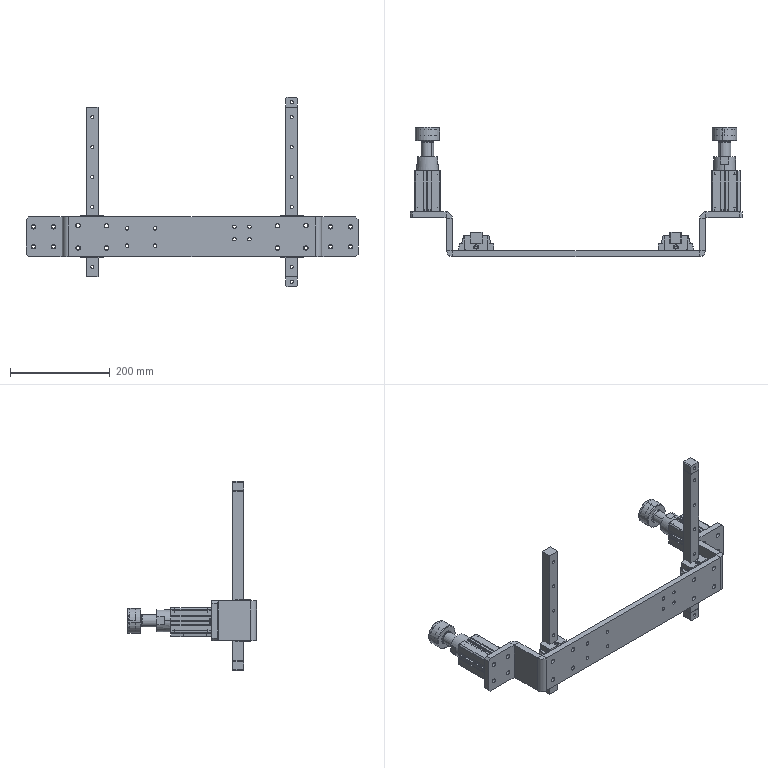Part | SolidWorks | features CompositeCurve 1 | 19 solids | 1058 faces | box 666 x 259.2 x 380 mm | volume 1864950 mm3 | plane 446 | cylinder 386 | torus 106 | cone 56 | sphere 56 | spline 8 | commonest cylinder face diameters 9 x40 11 x36 9.5 x32 6.6 x28 6.8 x20 5 x16